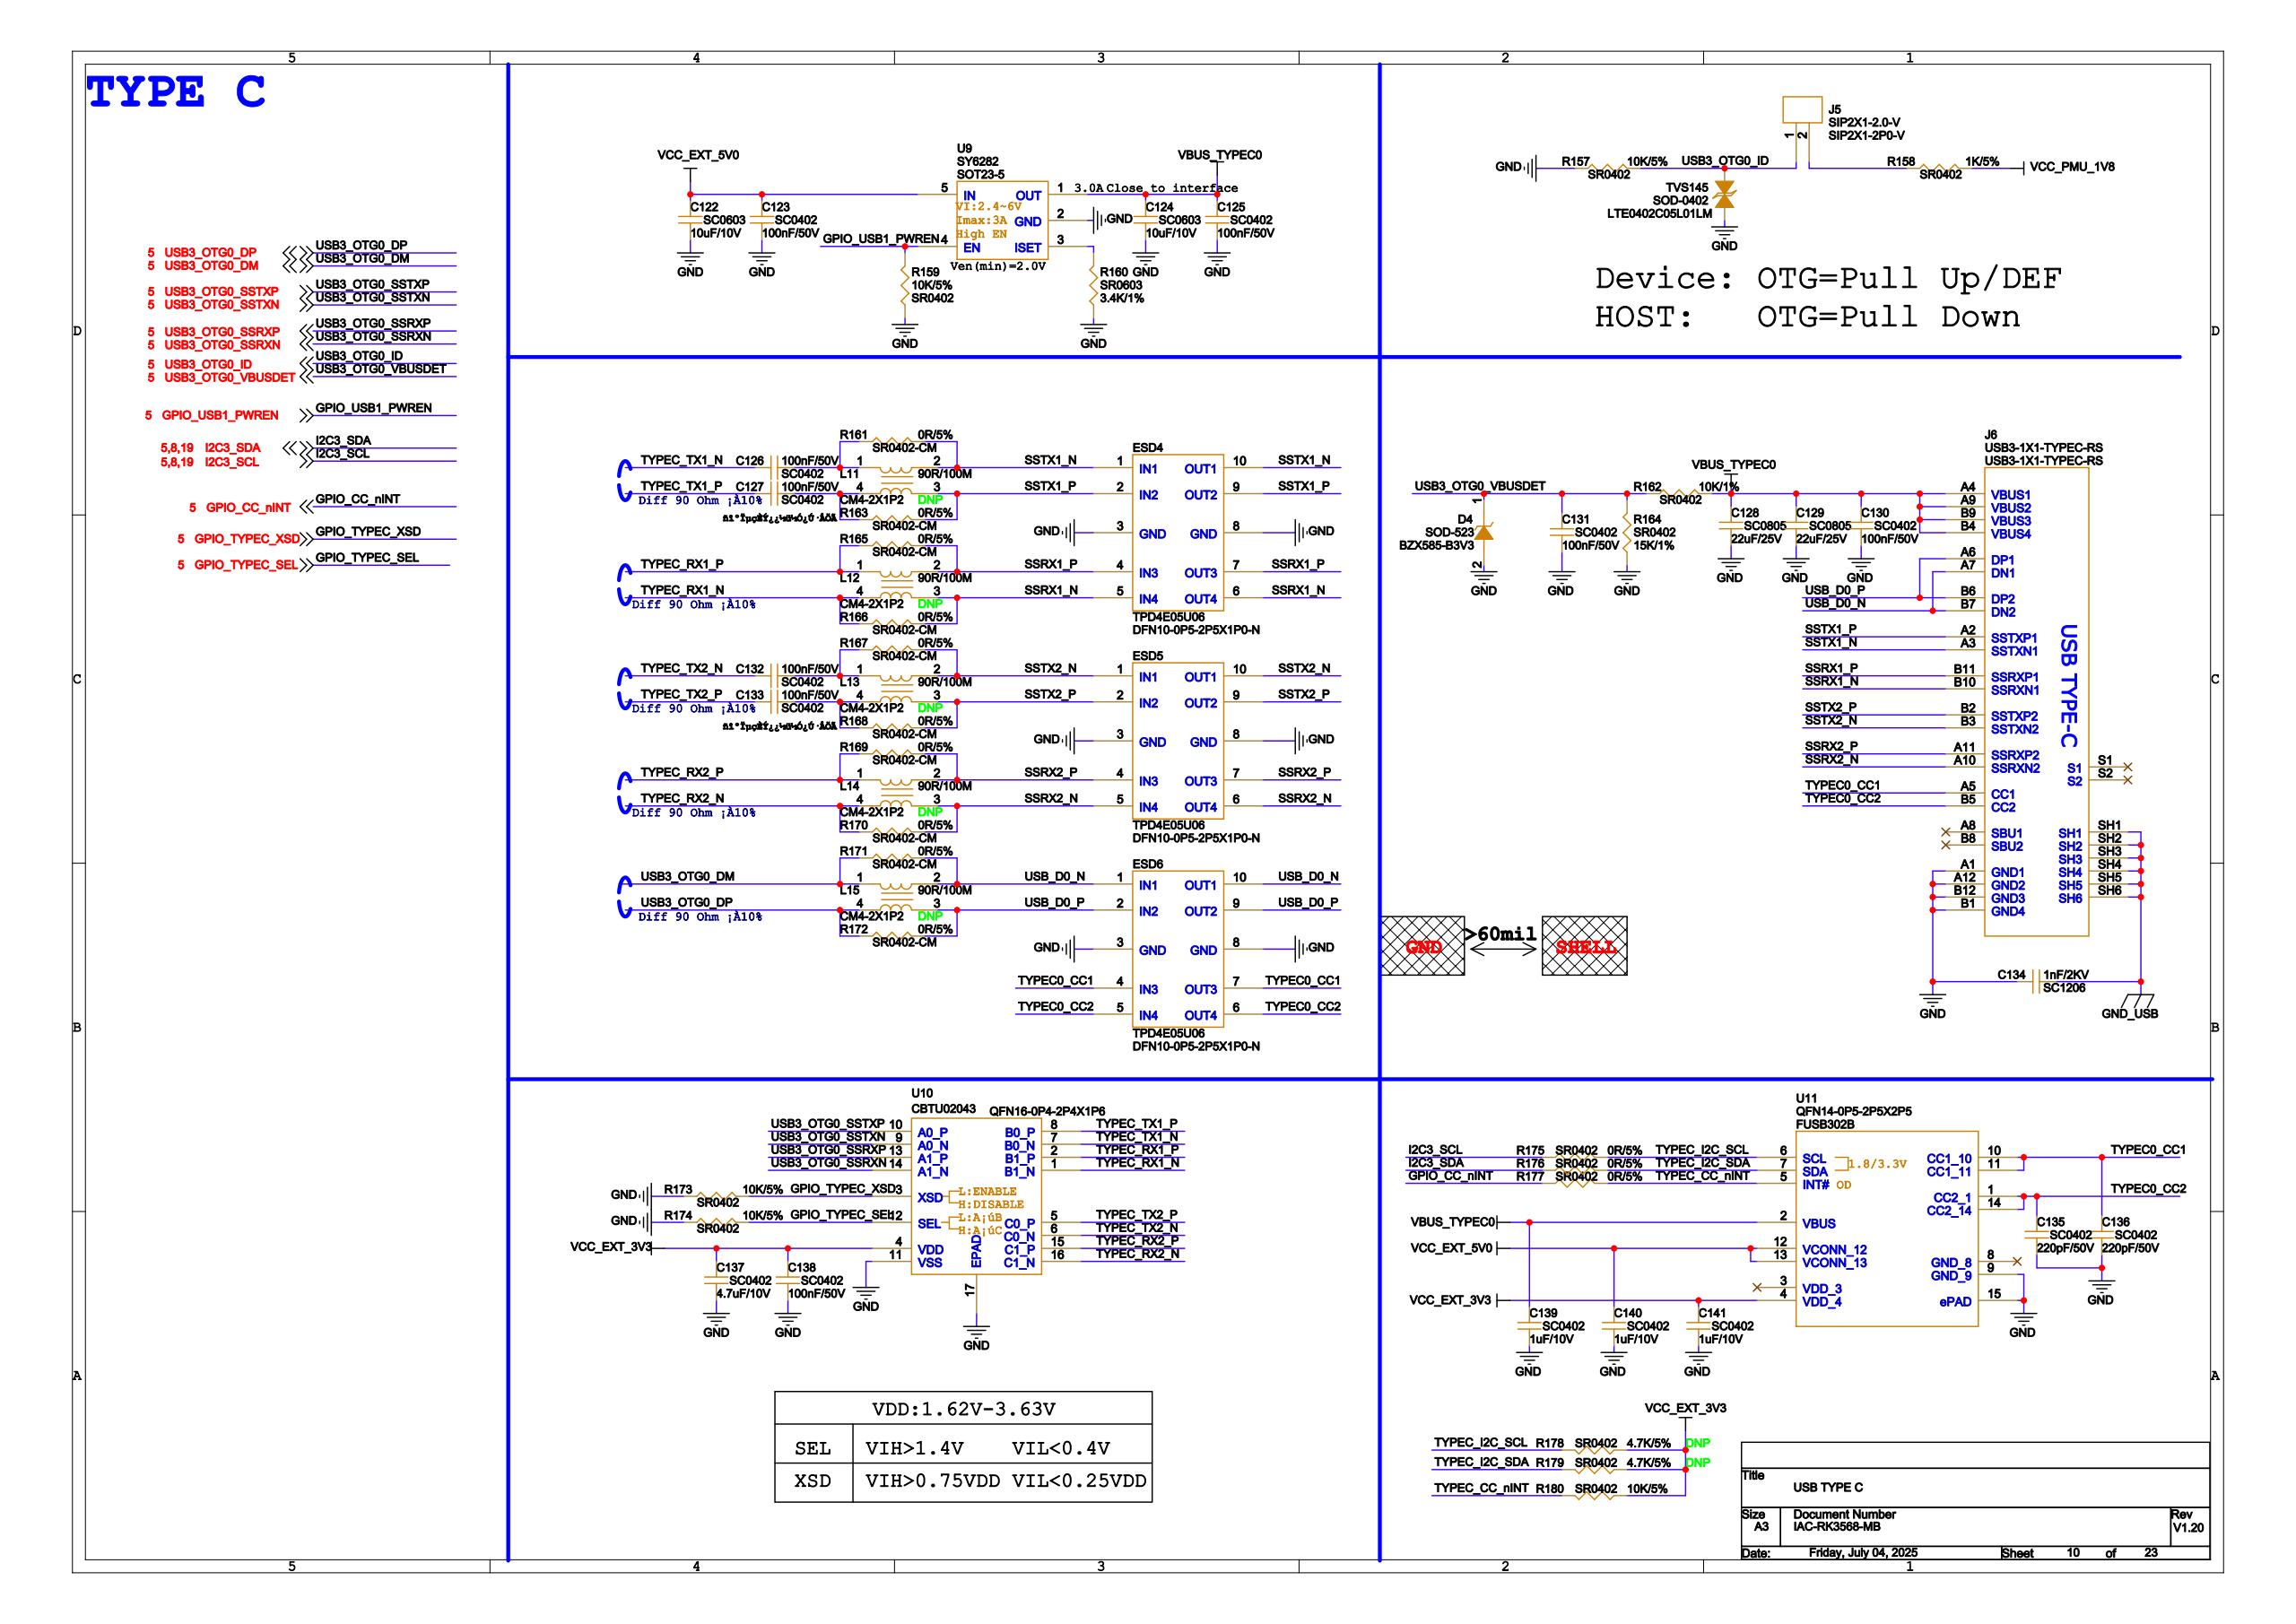Circuit board | Cadence Allegro | 1138 parts | 722 nets | one sheet of the schematic
Parts on this sheet (reference | value | footprint):
C122 | 10uF/10V | SC0603
C123 | 100nF/50V | SC0402
C124 | 10uF/10V | SC0603
C125 | 100nF/50V | SC0402
C126 | 100nF/50V | SC0402
C127 | 100nF/50V | SC0402
C128 | 22uF/25V | SC0805
C129 | 22uF/25V | SC0805
C130 | 100nF/50V | SC0402
C131 | 100nF/50V | SC0402
C132 | 100nF/50V | SC0402
C133 | 100nF/50V | SC0402
C134 | 1nF/2KV | SC1206
C135 | 220pF/50V | SC0402
C136 | 220pF/50V | SC0402
C137 | 4.7uF/10V | SC0402
C138 | 100nF/50V | SC0402
C139 | 1uF/10V | SC0402
C140 | 1uF/10V | SC0402
C141 | 1uF/10V | SC0402
D4 | BZX585-B3V3 | SOD-523
ESD4 | TPD4E05U06 | DFN10-0P5-2P5X1P0-N
ESD5 | TPD4E05U06 | DFN10-0P5-2P5X1P0-N
ESD6 | TPD4E05U06 | DFN10-0P5-2P5X1P0-N
J5 | SIP2X1-2.0-V | SIP2X1-2P0-V
J6 | USB3-1X1-TYPEC-RS | USB3-1X1-TYPEC-RS
L11 | 90R/100M | CM4-2X1P2
L12 | 90R/100M | CM4-2X1P2
L13 | 90R/100M | CM4-2X1P2
L14 | 90R/100M | CM4-2X1P2
L15 | 90R/100M | CM4-2X1P2
R157 | 10K/5% | SR0402
R158 | 1K/5% | SR0402
R159 | 10K/5% | SR0402
R160 | 3.4K/1% | SR0603
R161 | 0R/5% | SR0402-CM
R162 | 10K/1% | SR0402
R163 | 0R/5% | SR0402-CM
R164 | 15K/1% | SR0402
R165 | 0R/5% | SR0402-CM
R166 | 0R/5% | SR0402-CM
R167 | 0R/5% | SR0402-CM
R168 | 0R/5% | SR0402-CM
R169 | 0R/5% | SR0402-CM
R170 | 0R/5% | SR0402-CM
R171 | 0R/5% | SR0402-CM
R172 | 0R/5% | SR0402-CM
R173 | 10K/5% | SR0402
R174 | 10K/5% | SR0402
R175 | 0R/5% | SR0402
R176 | 0R/5% | SR0402
R177 | 0R/5% | SR0402
R178 | 4.7K/5% | SR0402
R179 | 4.7K/5% | SR0402
R180 | 10K/5% | SR0402
TVS145 | LTE0402C05L01LM | SOD-0402
U9 | SY6282 | SOT23-5
U10 | CBTU02043 | QFN16-0P4-2P4X1P6
U11 | FUSB302B | QFN14-0P5-2P5X2P5
Nets of these parts (net: part-pin ...):
VCC_EXT_5V0: C122-1 C123-1 C140-1 U9-5 U11-12 U11-13
VCC_EXT_3V3: C137-1 C138-1 C141-1 R178-2 R179-2 R180-2 U10-4 U11-4
GND: C122-2 C123-2 C124-2 C125-2 C128-2 C129-2 C130-2 C131-2 C134-1 C135-2 C136-2 C137-2 C138-2 C139-2 C140-2 C141-2 D4-2 ESD4-3 ESD4-8 ESD5-3 ESD5-8 ESD6-3 ESD6-8 R157-2 R159-1 R160-1 R164-1 R173-1 R174-1 TVS145-1 U9-2 U10-11 U10-17 U11-9 U11-15 J6-A1 J6-A12 J6-B1 J6-B12
TYPEC_RX2_P: L14-1 R169-1 U10-15
SSRX2_P: ESD5-4 ESD5-7 L14-2 R169-2 J6-A11
N98871: C126-2 L11-1 R161-1
SSTX1_N: ESD4-1 ESD4-10 L11-2 R161-2 J6-A3
N98875: C127-2 L11-4 R163-1
SSTX1_P: ESD4-2 ESD4-9 L11-3 R163-2 J6-A2
TYPEC_RX1_P: L12-1 R165-1 U10-2
SSRX1_P: ESD4-4 ESD4-7 L12-2 R165-2 J6-B11
TYPEC_RX1_N: L12-4 R166-1 U10-1
SSRX1_N: ESD4-5 ESD4-6 L12-3 R166-2 J6-B10
N99119: C132-2 L13-1 R167-1
SSTX2_N: ESD5-1 ESD5-10 L13-2 R167-2 J6-B3
N99079: C133-2 L13-4 R168-1
SSTX2_P: ESD5-2 ESD5-9 L13-3 R168-2 J6-B2
TYPEC_RX2_N: L14-4 R170-1 U10-16
SSRX2_N: ESD5-5 ESD5-6 L14-3 R170-2 J6-A10
USB3_OTG0_DM: L15-1 R171-1
USB_D0_N: ESD6-1 ESD6-10 L15-2 R171-2 J6-A7 J6-B7
USB3_OTG0_DP: L15-4 R172-1
USB_D0_P: ESD6-2 ESD6-9 L15-3 R172-2 J6-A6 J6-B6
TYPEC0_CC1: C136-1 ESD6-4 ESD6-7 U11-10 U11-11 J6-A5
TYPEC0_CC2: C135-1 ESD6-5 ESD6-6 U11-1 U11-14 J6-B5
TYPEC_CC_NINT: R177-1 R180-1 U11-5
TYPEC_I2C_SCL: R175-1 R178-1 U11-6
TYPEC_I2C_SDA: R176-1 R179-1 U11-7
VBUS_TYPEC0: C124-1 C125-1 C128-1 C129-1 C130-1 C139-1 R162-2 U9-1 U11-2 J6-A4 J6-A9 J6-B4 J6-B9
GND_USB: C134-2 J6-SH1 J6-SH2 J6-SH3 J6-SH4 J6-SH5 J6-SH6
USB3_OTG0_VBUSDET: C131-1 D4-1 R162-1 R164-2
USB3_OTG0_ID: J5-1 R157-1 TVS145-2
N99943: J5-2 R158-1
N101069: R160-2 U9-3
GPIO_CC_NINT: R177-2
GPIO_TYPEC_XSD: R173-2 U10-3
GPIO_USB1_PWREN: R159-2 U9-4
GPIO_TYPEC_SEL: R174-2 U10-12
I2C3_SCL: R175-2
I2C3_SDA: R176-2
USB3_OTG0_SSRXN: U10-14
USB3_OTG0_SSRXP: U10-13
USB3_OTG0_SSTXN: U10-9
USB3_OTG0_SSTXP: U10-10
VCC_PMU_1V8: R158-2
TYPEC_TX1_N: C126-1 U10-7
TYPEC_TX1_P: C127-1 U10-8
TYPEC_TX2_N: C132-1 U10-6
TYPEC_TX2_P: C133-1 U10-5